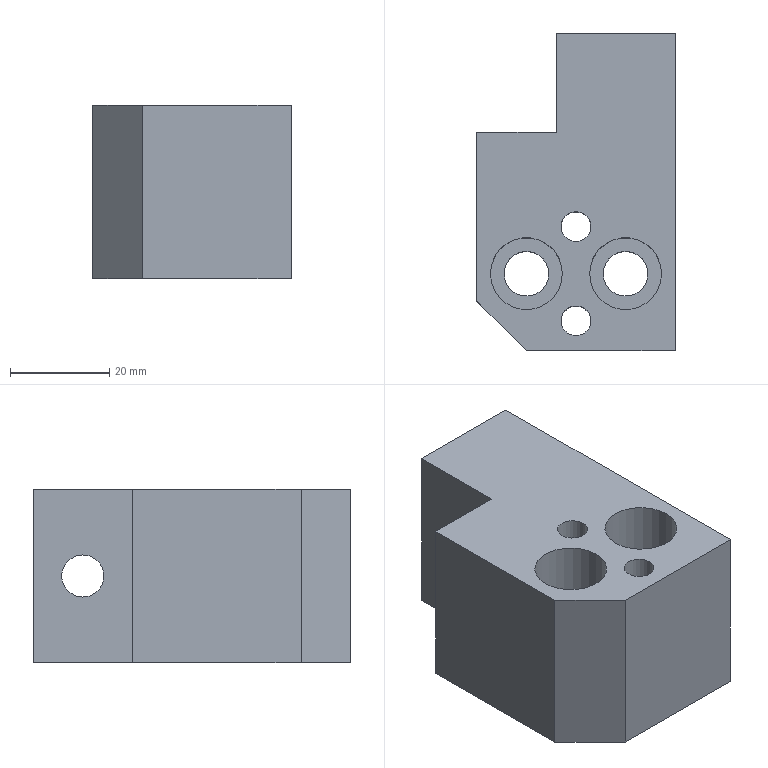Part | NX | features solid 2 | 1 solid | 18 faces | box 40 x 64 x 35 mm | volume 66622 mm3 | plane 11 | cylinder 7 | commonest cylinder face diameters 6.001 x2 9 x2 14.5 x2 8.5 x1
STEP:
#1=CARTESIAN_POINT('',(3985.,-494.5,70.5));
#2=VERTEX_POINT('',#1);
#3=CARTESIAN_POINT('',(3955.,-494.5,70.5));
#4=VERTEX_POINT('',#3);
#5=CARTESIAN_POINT('',(3982.5,-494.5,70.5));
#6=DIRECTION('',(-1.,0.,0.));
#7=VECTOR('',#6,1000.);
#8=LINE('',#5,#7);
#9=EDGE_CURVE('',#2,#4,#8,.T.);
#10=ORIENTED_EDGE('',*,*,#9,.T.);
#11=CARTESIAN_POINT('',(3945.,-484.5,70.5));
#12=VERTEX_POINT('',#11);
#13=CARTESIAN_POINT('',(3931.5,-471.,70.5));
#14=DIRECTION('',(-0.7071,0.7071,0.));
#15=VECTOR('',#14,1000.);
#16=LINE('',#13,#15);
#17=EDGE_CURVE('',#4,#12,#16,.T.);
#18=ORIENTED_EDGE('',*,*,#17,.T.);
#19=CARTESIAN_POINT('',(3945.,-450.5,70.5));
#20=VERTEX_POINT('',#19);
#21=CARTESIAN_POINT('',(3945.,-420.,70.5));
#22=DIRECTION('',(0.,1.,0.));
#23=VECTOR('',#22,1000.);
#24=LINE('',#21,#23);
#25=EDGE_CURVE('',#12,#20,#24,.T.);
#26=ORIENTED_EDGE('',*,*,#25,.T.);
#27=CARTESIAN_POINT('',(3961.,-450.5,70.5));
#28=VERTEX_POINT('',#27);
#29=CARTESIAN_POINT('',(3982.5,-450.5,70.5));
#30=DIRECTION('',(1.,0.,0.));
#31=VECTOR('',#30,1000.);
#32=LINE('',#29,#31);
#33=EDGE_CURVE('',#20,#28,#32,.T.);
#34=ORIENTED_EDGE('',*,*,#33,.T.);
#35=CARTESIAN_POINT('',(3961.,-430.5,70.5));
#36=VERTEX_POINT('',#35);
#37=CARTESIAN_POINT('',(3961.,-432.,70.5));
#38=DIRECTION('',(0.,1.,0.));
#39=VECTOR('',#38,1000.);
#40=LINE('',#37,#39);
#41=EDGE_CURVE('',#28,#36,#40,.T.);
#42=ORIENTED_EDGE('',*,*,#41,.T.);
#43=CARTESIAN_POINT('',(3985.,-430.5,70.5));
#44=VERTEX_POINT('',#43);
#45=CARTESIAN_POINT('',(3979.,-430.5,70.5));
#46=DIRECTION('',(1.,0.,0.));
#47=VECTOR('',#46,1000.);
#48=LINE('',#45,#47);
#49=EDGE_CURVE('',#36,#44,#48,.T.);
#50=ORIENTED_EDGE('',*,*,#49,.T.);
#51=CARTESIAN_POINT('',(3985.,-401.5,70.5));
#52=DIRECTION('',(0.,1.,0.));
#53=VECTOR('',#52,1000.);
#54=LINE('',#51,#53);
#55=EDGE_CURVE('',#2,#44,#54,.T.);
#56=ORIENTED_EDGE('',*,*,#55,.F.);
#57=EDGE_LOOP('',(#10,#18,#26,#34,#42,#50,#56));
#58=FACE_BOUND('',#57,.T.);
#59=CARTESIAN_POINT('',(3950.5,-479.,70.5));
#60=VERTEX_POINT('',#59);
#61=CARTESIAN_POINT('',(3955.,-479.,70.5));
#62=DIRECTION('',(0.,0.,-1.));
#63=DIRECTION('',(-1.,0.,0.));
#64=AXIS2_PLACEMENT_3D('',#61,#62,#63);
#65=CIRCLE('',#64,4.5);
#66=EDGE_CURVE('',#60,#60,#65,.T.);
#67=ORIENTED_EDGE('',*,*,#66,.F.);
#68=EDGE_LOOP('',(#67));
#69=FACE_BOUND('',#68,.T.);
#70=CARTESIAN_POINT('',(3970.5,-479.,70.5));
#71=VERTEX_POINT('',#70);
#72=CARTESIAN_POINT('',(3975.,-479.,70.5));
#73=DIRECTION('',(0.,0.,1.));
#74=DIRECTION('',(-1.,0.,0.));
#75=AXIS2_PLACEMENT_3D('',#72,#73,#74);
#76=CIRCLE('',#75,4.5);
#77=EDGE_CURVE('',#71,#71,#76,.T.);
#78=ORIENTED_EDGE('',*,*,#77,.T.);
#79=EDGE_LOOP('',(#78));
#80=FACE_BOUND('',#79,.T.);
#81=CARTESIAN_POINT('',(3968.001,-469.5,70.5));
#82=VERTEX_POINT('',#81);
#83=CARTESIAN_POINT('',(3965.,-469.5,70.5));
#84=DIRECTION('',(0.,0.,-1.));
#85=DIRECTION('',(1.,0.,0.));
#86=AXIS2_PLACEMENT_3D('',#83,#84,#85);
#87=CIRCLE('',#86,3.001);
#88=EDGE_CURVE('',#82,#82,#87,.T.);
#89=ORIENTED_EDGE('',*,*,#88,.F.);
#90=EDGE_LOOP('',(#89));
#91=FACE_BOUND('',#90,.T.);
#92=CARTESIAN_POINT('',(3968.001,-488.5,70.5));
#93=VERTEX_POINT('',#92);
#94=CARTESIAN_POINT('',(3965.,-488.5,70.5));
#95=DIRECTION('',(0.,0.,1.));
#96=DIRECTION('',(1.,0.,0.));
#97=AXIS2_PLACEMENT_3D('',#94,#95,#96);
#98=CIRCLE('',#97,3.001);
#99=EDGE_CURVE('',#93,#93,#98,.T.);
#100=ORIENTED_EDGE('',*,*,#99,.T.);
#101=EDGE_LOOP('',(#100));
#102=FACE_BOUND('',#101,.T.);
#103=CARTESIAN_POINT('',(3982.5,-420.,70.5));
#104=DIRECTION('',(0.,0.,-1.));
#105=DIRECTION('',(0.,1.,0.));
#106=AXIS2_PLACEMENT_3D('',#103,#104,#105);
#107=PLANE('',#106);
#108=ADVANCED_FACE('',(#58,#69,#80,#91,#102),#107,.T.);
#109=CARTESIAN_POINT('',(3968.001,-488.5,105.5));
#110=VERTEX_POINT('',#109);
#111=CARTESIAN_POINT('',(3965.,-488.5,105.5));
#112=DIRECTION('',(0.,0.,1.));
#113=DIRECTION('',(1.,0.,0.));
#114=AXIS2_PLACEMENT_3D('',#111,#112,#113);
#115=CIRCLE('',#114,3.001);
#116=EDGE_CURVE('',#110,#110,#115,.T.);
#117=ORIENTED_EDGE('',*,*,#116,.F.);
#118=EDGE_LOOP('',(#117));
#119=FACE_BOUND('',#118,.T.);
#120=CARTESIAN_POINT('',(3945.,-450.5,105.5));
#121=VERTEX_POINT('',#120);
#122=CARTESIAN_POINT('',(3945.,-484.5,105.5));
#123=VERTEX_POINT('',#122);
#124=CARTESIAN_POINT('',(3945.,-420.,105.5));
#125=DIRECTION('',(0.,-1.,0.));
#126=VECTOR('',#125,1000.);
#127=LINE('',#124,#126);
#128=EDGE_CURVE('',#121,#123,#127,.T.);
#129=ORIENTED_EDGE('',*,*,#128,.T.);
#130=CARTESIAN_POINT('',(3955.,-494.5,105.5));
#131=VERTEX_POINT('',#130);
#132=CARTESIAN_POINT('',(3931.5,-471.,105.5));
#133=DIRECTION('',(0.7071,-0.7071,0.));
#134=VECTOR('',#133,1000.);
#135=LINE('',#132,#134);
#136=EDGE_CURVE('',#123,#131,#135,.T.);
#137=ORIENTED_EDGE('',*,*,#136,.T.);
#138=CARTESIAN_POINT('',(3985.,-494.5,105.5));
#139=VERTEX_POINT('',#138);
#140=CARTESIAN_POINT('',(3982.5,-494.5,105.5));
#141=DIRECTION('',(1.,0.,0.));
#142=VECTOR('',#141,1000.);
#143=LINE('',#140,#142);
#144=EDGE_CURVE('',#131,#139,#143,.T.);
#145=ORIENTED_EDGE('',*,*,#144,.T.);
#146=CARTESIAN_POINT('',(3985.,-430.5,105.5));
#147=VERTEX_POINT('',#146);
#148=CARTESIAN_POINT('',(3985.,-401.5,105.5));
#149=DIRECTION('',(0.,-1.,0.));
#150=VECTOR('',#149,1000.);
#151=LINE('',#148,#150);
#152=EDGE_CURVE('',#147,#139,#151,.T.);
#153=ORIENTED_EDGE('',*,*,#152,.F.);
#154=CARTESIAN_POINT('',(3961.,-430.5,105.5));
#155=VERTEX_POINT('',#154);
#156=CARTESIAN_POINT('',(3979.,-430.5,105.5));
#157=DIRECTION('',(-1.,0.,0.));
#158=VECTOR('',#157,1000.);
#159=LINE('',#156,#158);
#160=EDGE_CURVE('',#147,#155,#159,.T.);
#161=ORIENTED_EDGE('',*,*,#160,.T.);
#162=CARTESIAN_POINT('',(3961.,-450.5,105.5));
#163=VERTEX_POINT('',#162);
#164=CARTESIAN_POINT('',(3961.,-432.,105.5));
#165=DIRECTION('',(0.,-1.,0.));
#166=VECTOR('',#165,1000.);
#167=LINE('',#164,#166);
#168=EDGE_CURVE('',#155,#163,#167,.T.);
#169=ORIENTED_EDGE('',*,*,#168,.T.);
#170=CARTESIAN_POINT('',(3982.5,-450.5,105.5));
#171=DIRECTION('',(-1.,0.,0.));
#172=VECTOR('',#171,1000.);
#173=LINE('',#170,#172);
#174=EDGE_CURVE('',#163,#121,#173,.T.);
#175=ORIENTED_EDGE('',*,*,#174,.T.);
#176=EDGE_LOOP('',(#129,#137,#145,#153,#161,#169,#175));
#177=FACE_BOUND('',#176,.T.);
#178=CARTESIAN_POINT('',(3962.25,-479.,105.5));
#179=VERTEX_POINT('',#178);
#180=CARTESIAN_POINT('',(3955.,-479.,105.5));
#181=DIRECTION('',(0.,0.,1.));
#182=DIRECTION('',(1.,0.,0.));
#183=AXIS2_PLACEMENT_3D('',#180,#181,#182);
#184=CIRCLE('',#183,7.25);
#185=EDGE_CURVE('',#179,#179,#184,.T.);
#186=ORIENTED_EDGE('',*,*,#185,.F.);
#187=EDGE_LOOP('',(#186));
#188=FACE_BOUND('',#187,.T.);
#189=CARTESIAN_POINT('',(3982.25,-479.,105.5));
#190=VERTEX_POINT('',#189);
#191=CARTESIAN_POINT('',(3975.,-479.,105.5));
#192=DIRECTION('',(0.,0.,-1.));
#193=DIRECTION('',(1.,0.,0.));
#194=AXIS2_PLACEMENT_3D('',#191,#192,#193);
#195=CIRCLE('',#194,7.25);
#196=EDGE_CURVE('',#190,#190,#195,.T.);
#197=ORIENTED_EDGE('',*,*,#196,.T.);
#198=EDGE_LOOP('',(#197));
#199=FACE_BOUND('',#198,.T.);
#200=CARTESIAN_POINT('',(3968.001,-469.5,105.5));
#201=VERTEX_POINT('',#200);
#202=CARTESIAN_POINT('',(3965.,-469.5,105.5));
#203=DIRECTION('',(0.,0.,-1.));
#204=DIRECTION('',(1.,0.,0.));
#205=AXIS2_PLACEMENT_3D('',#202,#203,#204);
#206=CIRCLE('',#205,3.001);
#207=EDGE_CURVE('',#201,#201,#206,.T.);
#208=ORIENTED_EDGE('',*,*,#207,.T.);
#209=EDGE_LOOP('',(#208));
#210=FACE_BOUND('',#209,.T.);
#211=CARTESIAN_POINT('',(3982.5,-420.,105.5));
#212=DIRECTION('',(0.,0.,1.));
#213=DIRECTION('',(0.,-1.,0.));
#214=AXIS2_PLACEMENT_3D('',#211,#212,#213);
#215=PLANE('',#214);
#216=ADVANCED_FACE('',(#119,#177,#188,#199,#210),#215,.T.);
#217=ORIENTED_EDGE('',*,*,#25,.F.);
#218=CARTESIAN_POINT('',(3945.,-484.5,88.));
#219=DIRECTION('',(0.,0.,1.));
#220=VECTOR('',#219,1000.);
#221=LINE('',#218,#220);
#222=EDGE_CURVE('',#12,#123,#221,.T.);
#223=ORIENTED_EDGE('',*,*,#222,.T.);
#224=ORIENTED_EDGE('',*,*,#128,.F.);
#225=CARTESIAN_POINT('',(3945.,-450.5,88.));
#226=DIRECTION('',(0.,0.,-1.));
#227=VECTOR('',#226,1000.);
#228=LINE('',#225,#227);
#229=EDGE_CURVE('',#121,#20,#228,.T.);
#230=ORIENTED_EDGE('',*,*,#229,.T.);
#231=EDGE_LOOP('',(#217,#223,#224,#230));
#232=FACE_BOUND('',#231,.T.);
#233=CARTESIAN_POINT('',(3945.,-488.993,88.));
#234=DIRECTION('',(-1.,0.,0.));
#235=DIRECTION('',(0.,1.,0.));
#236=AXIS2_PLACEMENT_3D('',#233,#234,#235);
#237=PLANE('',#236);
#238=ADVANCED_FACE('',(#232),#237,.T.);
#239=ORIENTED_EDGE('',*,*,#144,.F.);
#240=CARTESIAN_POINT('',(3955.,-494.5,88.));
#241=DIRECTION('',(0.,0.,-1.));
#242=VECTOR('',#241,1000.);
#243=LINE('',#240,#242);
#244=EDGE_CURVE('',#131,#4,#243,.T.);
#245=ORIENTED_EDGE('',*,*,#244,.T.);
#246=ORIENTED_EDGE('',*,*,#9,.F.);
#247=CARTESIAN_POINT('',(3985.,-494.5,88.));
#248=DIRECTION('',(0.,0.,-1.));
#249=VECTOR('',#248,1000.);
#250=LINE('',#247,#249);
#251=EDGE_CURVE('',#139,#2,#250,.T.);
#252=ORIENTED_EDGE('',*,*,#251,.F.);
#253=EDGE_LOOP('',(#239,#245,#246,#252));
#254=FACE_BOUND('',#253,.T.);
#255=CARTESIAN_POINT('',(3966.75,-494.5,88.));
#256=DIRECTION('',(0.,-1.,0.));
#257=DIRECTION('',(0.,0.,-1.));
#258=AXIS2_PLACEMENT_3D('',#255,#256,#257);
#259=PLANE('',#258);
#260=ADVANCED_FACE('',(#254),#259,.T.);
#261=ORIENTED_EDGE('',*,*,#174,.F.);
#262=CARTESIAN_POINT('',(3961.,-450.5,88.));
#263=DIRECTION('',(0.,0.,1.));
#264=VECTOR('',#263,1000.);
#265=LINE('',#262,#264);
#266=EDGE_CURVE('',#28,#163,#265,.T.);
#267=ORIENTED_EDGE('',*,*,#266,.F.);
#268=ORIENTED_EDGE('',*,*,#33,.F.);
#269=ORIENTED_EDGE('',*,*,#229,.F.);
#270=EDGE_LOOP('',(#261,#267,#268,#269));
#271=FACE_BOUND('',#270,.T.);
#272=CARTESIAN_POINT('',(3985.,-450.5,88.));
#273=DIRECTION('',(0.,-1.,0.));
#274=DIRECTION('',(-1.,0.,0.));
#275=AXIS2_PLACEMENT_3D('',#272,#273,#274);
#276=PLANE('',#275);
#277=ADVANCED_FACE('',(#271),#276,.F.);
#278=ORIENTED_EDGE('',*,*,#152,.T.);
#279=ORIENTED_EDGE('',*,*,#251,.T.);
#280=ORIENTED_EDGE('',*,*,#55,.T.);
#281=CARTESIAN_POINT('',(3985.,-430.5,88.));
#282=DIRECTION('',(0.,0.,1.));
#283=VECTOR('',#282,1000.);
#284=LINE('',#281,#283);
#285=EDGE_CURVE('',#44,#147,#284,.T.);
#286=ORIENTED_EDGE('',*,*,#285,.T.);
#287=EDGE_LOOP('',(#278,#279,#280,#286));
#288=FACE_BOUND('',#287,.T.);
#289=CARTESIAN_POINT('',(3985.,-440.5,83.75));
#290=VERTEX_POINT('',#289);
#291=CARTESIAN_POINT('',(3985.,-440.5,88.));
#292=DIRECTION('',(1.,0.,0.));
#293=DIRECTION('',(0.,0.,-1.));
#294=AXIS2_PLACEMENT_3D('',#291,#292,#293);
#295=CIRCLE('',#294,4.25);
#296=EDGE_CURVE('',#290,#290,#295,.T.);
#297=ORIENTED_EDGE('',*,*,#296,.F.);
#298=EDGE_LOOP('',(#297));
#299=FACE_BOUND('',#298,.T.);
#300=CARTESIAN_POINT('',(3985.,-401.5,88.));
#301=DIRECTION('',(1.,0.,0.));
#302=DIRECTION('',(0.,0.,-1.));
#303=AXIS2_PLACEMENT_3D('',#300,#301,#302);
#304=PLANE('',#303);
#305=ADVANCED_FACE('',(#288,#299),#304,.T.);
#306=CARTESIAN_POINT('',(3970.5,-479.,94.5));
#307=VERTEX_POINT('',#306);
#308=CARTESIAN_POINT('',(3975.,-479.,94.5));
#309=DIRECTION('',(0.,0.,-1.));
#310=DIRECTION('',(-1.,0.,0.));
#311=AXIS2_PLACEMENT_3D('',#308,#309,#310);
#312=CIRCLE('',#311,4.5);
#313=EDGE_CURVE('',#307,#307,#312,.T.);
#314=ORIENTED_EDGE('',*,*,#313,.F.);
#315=EDGE_LOOP('',(#314));
#316=FACE_BOUND('',#315,.T.);
#317=ORIENTED_EDGE('',*,*,#77,.F.);
#318=EDGE_LOOP('',(#317));
#319=FACE_BOUND('',#318,.T.);
#320=CARTESIAN_POINT('',(3975.,-479.,105.5));
#321=DIRECTION('',(0.,0.,-1.));
#322=DIRECTION('',(1.,0.,0.));
#323=AXIS2_PLACEMENT_3D('',#320,#321,#322);
#324=CYLINDRICAL_SURFACE('',#323,4.5);
#325=ADVANCED_FACE('',(#316,#319),#324,.F.);
#326=ORIENTED_EDGE('',*,*,#313,.T.);
#327=EDGE_LOOP('',(#326));
#328=FACE_BOUND('',#327,.T.);
#329=CARTESIAN_POINT('',(3967.75,-479.,94.5));
#330=VERTEX_POINT('',#329);
#331=CARTESIAN_POINT('',(3975.,-479.,94.5));
#332=DIRECTION('',(0.,0.,-1.));
#333=DIRECTION('',(-1.,0.,0.));
#334=AXIS2_PLACEMENT_3D('',#331,#332,#333);
#335=CIRCLE('',#334,7.25);
#336=EDGE_CURVE('',#330,#330,#335,.T.);
#337=ORIENTED_EDGE('',*,*,#336,.F.);
#338=EDGE_LOOP('',(#337));
#339=FACE_BOUND('',#338,.T.);
#340=CARTESIAN_POINT('',(3975.,-479.,94.5));
#341=DIRECTION('',(0.,0.,-1.));
#342=DIRECTION('',(-1.,0.,0.));
#343=AXIS2_PLACEMENT_3D('',#340,#341,#342);
#344=PLANE('',#343);
#345=ADVANCED_FACE('',(#328,#339),#344,.F.);
#346=ORIENTED_EDGE('',*,*,#336,.T.);
#347=EDGE_LOOP('',(#346));
#348=FACE_BOUND('',#347,.T.);
#349=ORIENTED_EDGE('',*,*,#196,.F.);
#350=EDGE_LOOP('',(#349));
#351=FACE_BOUND('',#350,.T.);
#352=CARTESIAN_POINT('',(3975.,-479.,105.5));
#353=DIRECTION('',(0.,0.,-1.));
#354=DIRECTION('',(1.,0.,0.));
#355=AXIS2_PLACEMENT_3D('',#352,#353,#354);
#356=CYLINDRICAL_SURFACE('',#355,7.25);
#357=ADVANCED_FACE('',(#348,#351),#356,.F.);
#358=CARTESIAN_POINT('',(3950.5,-479.,94.5));
#359=VERTEX_POINT('',#358);
#360=CARTESIAN_POINT('',(3955.,-479.,94.5));
#361=DIRECTION('',(0.,0.,1.));
#362=DIRECTION('',(-1.,0.,0.));
#363=AXIS2_PLACEMENT_3D('',#360,#361,#362);
#364=CIRCLE('',#363,4.5);
#365=EDGE_CURVE('',#359,#359,#364,.T.);
#366=ORIENTED_EDGE('',*,*,#365,.T.);
#367=EDGE_LOOP('',(#366));
#368=FACE_BOUND('',#367,.T.);
#369=ORIENTED_EDGE('',*,*,#66,.T.);
#370=EDGE_LOOP('',(#369));
#371=FACE_BOUND('',#370,.T.);
#372=CARTESIAN_POINT('',(3955.,-479.,105.5));
#373=DIRECTION('',(0.,0.,-1.));
#374=DIRECTION('',(-1.,0.,0.));
#375=AXIS2_PLACEMENT_3D('',#372,#373,#374);
#376=CYLINDRICAL_SURFACE('',#375,4.5);
#377=ADVANCED_FACE('',(#368,#371),#376,.F.);
#378=ORIENTED_EDGE('',*,*,#365,.F.);
#379=EDGE_LOOP('',(#378));
#380=FACE_BOUND('',#379,.T.);
#381=CARTESIAN_POINT('',(3947.75,-479.,94.5));
#382=VERTEX_POINT('',#381);
#383=CARTESIAN_POINT('',(3955.,-479.,94.5));
#384=DIRECTION('',(0.,0.,1.));
#385=DIRECTION('',(-1.,0.,0.));
#386=AXIS2_PLACEMENT_3D('',#383,#384,#385);
#387=CIRCLE('',#386,7.25);
#388=EDGE_CURVE('',#382,#382,#387,.T.);
#389=ORIENTED_EDGE('',*,*,#388,.T.);
#390=EDGE_LOOP('',(#389));
#391=FACE_BOUND('',#390,.T.);
#392=CARTESIAN_POINT('',(3952.,-479.,94.5));
#393=DIRECTION('',(0.,0.,-1.));
#394=DIRECTION('',(1.,0.,0.));
#395=AXIS2_PLACEMENT_3D('',#392,#393,#394);
#396=PLANE('',#395);
#397=ADVANCED_FACE('',(#380,#391),#396,.F.);
#398=ORIENTED_EDGE('',*,*,#388,.F.);
#399=EDGE_LOOP('',(#398));
#400=FACE_BOUND('',#399,.T.);
#401=ORIENTED_EDGE('',*,*,#185,.T.);
#402=EDGE_LOOP('',(#401));
#403=FACE_BOUND('',#402,.T.);
#404=CARTESIAN_POINT('',(3955.,-479.,105.5));
#405=DIRECTION('',(0.,0.,-1.));
#406=DIRECTION('',(-1.,0.,0.));
#407=AXIS2_PLACEMENT_3D('',#404,#405,#406);
#408=CYLINDRICAL_SURFACE('',#407,7.25);
#409=ADVANCED_FACE('',(#400,#403),#408,.F.);
#410=ORIENTED_EDGE('',*,*,#296,.T.);
#411=EDGE_LOOP('',(#410));
#412=FACE_BOUND('',#411,.T.);
#413=CARTESIAN_POINT('',(3961.,-440.5,83.75));
#414=VERTEX_POINT('',#413);
#415=CARTESIAN_POINT('',(3961.,-440.5,88.));
#416=DIRECTION('',(1.,0.,0.));
#417=DIRECTION('',(0.,0.,-1.));
#418=AXIS2_PLACEMENT_3D('',#415,#416,#417);
#419=CIRCLE('',#418,4.25);
#420=EDGE_CURVE('',#414,#414,#419,.T.);
#421=ORIENTED_EDGE('',*,*,#420,.F.);
#422=EDGE_LOOP('',(#421));
#423=FACE_BOUND('',#422,.T.);
#424=CARTESIAN_POINT('',(3975.,-440.5,88.));
#425=DIRECTION('',(-1.,0.,0.));
#426=DIRECTION('',(0.,1.,0.));
#427=AXIS2_PLACEMENT_3D('',#424,#425,#426);
#428=CYLINDRICAL_SURFACE('',#427,4.25);
#429=ADVANCED_FACE('',(#412,#423),#428,.F.);
#430=CARTESIAN_POINT('',(3961.,-430.5,353.));
#431=DIRECTION('',(0.,0.,-1.));
#432=VECTOR('',#431,1000.);
#433=LINE('',#430,#432);
#434=EDGE_CURVE('',#155,#36,#433,.T.);
#435=ORIENTED_EDGE('',*,*,#434,.F.);
#436=ORIENTED_EDGE('',*,*,#160,.F.);
#437=ORIENTED_EDGE('',*,*,#285,.F.);
#438=ORIENTED_EDGE('',*,*,#49,.F.);
#439=EDGE_LOOP('',(#435,#436,#437,#438));
#440=FACE_BOUND('',#439,.T.);
#441=CARTESIAN_POINT('',(3979.,-430.5,353.));
#442=DIRECTION('',(0.,-1.,0.));
#443=DIRECTION('',(-1.,0.,0.));
#444=AXIS2_PLACEMENT_3D('',#441,#442,#443);
#445=PLANE('',#444);
#446=ADVANCED_FACE('',(#440),#445,.F.);
#447=ORIENTED_EDGE('',*,*,#266,.T.);
#448=ORIENTED_EDGE('',*,*,#168,.F.);
#449=ORIENTED_EDGE('',*,*,#434,.T.);
#450=ORIENTED_EDGE('',*,*,#41,.F.);
#451=EDGE_LOOP('',(#447,#448,#449,#450));
#452=FACE_BOUND('',#451,.T.);
#453=ORIENTED_EDGE('',*,*,#420,.T.);
#454=EDGE_LOOP('',(#453));
#455=FACE_BOUND('',#454,.T.);
#456=CARTESIAN_POINT('',(3961.,-413.5,88.));
#457=DIRECTION('',(1.,0.,0.));
#458=DIRECTION('',(0.,0.,-1.));
#459=AXIS2_PLACEMENT_3D('',#456,#457,#458);
#460=PLANE('',#459);
#461=ADVANCED_FACE('',(#452,#455),#460,.F.);
#462=ORIENTED_EDGE('',*,*,#136,.F.);
#463=ORIENTED_EDGE('',*,*,#222,.F.);
#464=ORIENTED_EDGE('',*,*,#17,.F.);
#465=ORIENTED_EDGE('',*,*,#244,.F.);
#466=EDGE_LOOP('',(#462,#463,#464,#465));
#467=FACE_BOUND('',#466,.T.);
#468=CARTESIAN_POINT('',(3955.,-494.5,88.));
#469=DIRECTION('',(0.7071,0.7071,0.));
#470=DIRECTION('',(0.,0.,1.));
#471=AXIS2_PLACEMENT_3D('',#468,#469,#470);
#472=PLANE('',#471);
#473=ADVANCED_FACE('',(#467),#472,.F.);
#474=ORIENTED_EDGE('',*,*,#207,.F.);
#475=EDGE_LOOP('',(#474));
#476=FACE_BOUND('',#475,.T.);
#477=ORIENTED_EDGE('',*,*,#88,.T.);
#478=EDGE_LOOP('',(#477));
#479=FACE_BOUND('',#478,.T.);
#480=CARTESIAN_POINT('',(3965.,-469.5,105.5));
#481=DIRECTION('',(0.,0.,-1.));
#482=DIRECTION('',(1.,0.,0.));
#483=AXIS2_PLACEMENT_3D('',#480,#481,#482);
#484=CYLINDRICAL_SURFACE('',#483,3.001);
#485=ADVANCED_FACE('',(#476,#479),#484,.F.);
#486=ORIENTED_EDGE('',*,*,#116,.T.);
#487=EDGE_LOOP('',(#486));
#488=FACE_BOUND('',#487,.T.);
#489=ORIENTED_EDGE('',*,*,#99,.F.);
#490=EDGE_LOOP('',(#489));
#491=FACE_BOUND('',#490,.T.);
#492=CARTESIAN_POINT('',(3965.,-488.5,105.5));
#493=DIRECTION('',(0.,0.,-1.));
#494=DIRECTION('',(1.,0.,0.));
#495=AXIS2_PLACEMENT_3D('',#492,#493,#494);
#496=CYLINDRICAL_SURFACE('',#495,3.001);
#497=ADVANCED_FACE('',(#488,#491),#496,.F.);
#498=CLOSED_SHELL('',(#108,#216,#238,#260,#277,#305,#325,#345,#357,#377,#397,#409,#429,#446,#461,#473,#485,#497));
#499=MANIFOLD_SOLID_BREP('',#498);
#500=(LENGTH_UNIT()NAMED_UNIT(*)SI_UNIT(.MILLI.,.METRE.));
#501=UNCERTAINTY_MEASURE_WITH_UNIT(LENGTH_MEASURE(0.00001),#500,'','');
#502=(NAMED_UNIT(*)PLANE_ANGLE_UNIT()SI_UNIT($,.RADIAN.));
#503=(NAMED_UNIT(*)SI_UNIT($,.STERADIAN.)SOLID_ANGLE_UNIT());
#504=(GEOMETRIC_REPRESENTATION_CONTEXT(3)GLOBAL_UNCERTAINTY_ASSIGNED_CONTEXT((#501))GLOBAL_UNIT_ASSIGNED_CONTEXT((#500,#502,#503))REPRESENTATION_CONTEXT('',''));
#505=ADVANCED_BREP_SHAPE_REPRESENTATION('',(#499),#504);